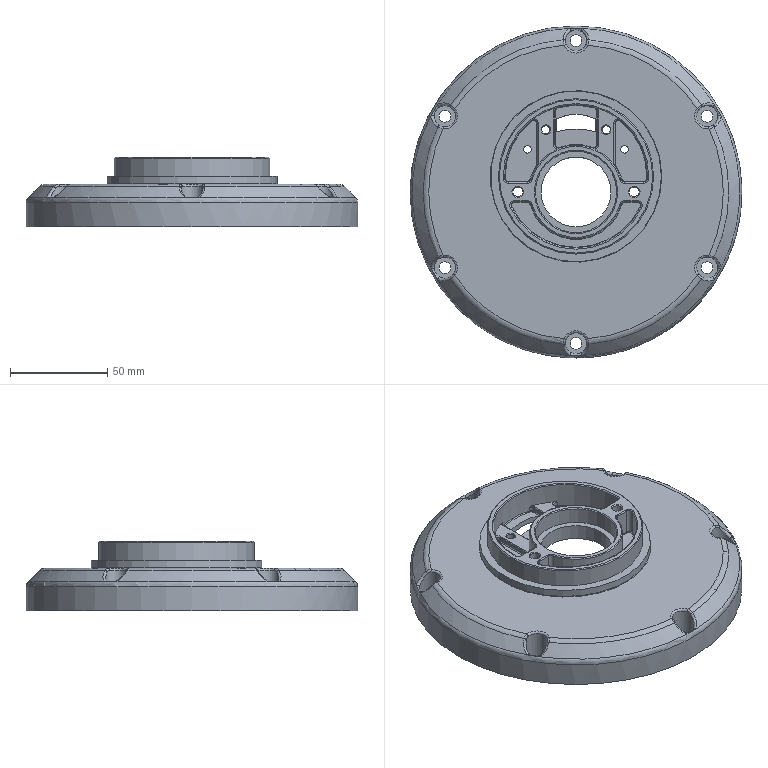NC program | NX | posted with a generic post | part box 171 x 171 x 36 mm
Lines 1 to 842 of 127321:
N10 G17 G21 G94 G90
(动态加工0.5 , TOOL : D12-L45)
N12 T01 M6
N14 G54
N16 G17 G0 G90 X-64.382 Y9.05 S4000 M3
N18 G43 Z20. H1
N20 Z-10.88
N22 G94 G1 X-64.242 Y8.994 Z-11.817 F2500.
N24 X-64.103 Y8.938 Z-12.188
N26 X-63.964 Y8.882 Z-12.46
N28 X-63.825 Y8.826 Z-12.68
N30 X-63.686 Y8.77 Z-12.864
N32 X-63.547 Y8.714 Z-13.022
N34 X-63.407 Y8.658 Z-13.16
N36 X-63.268 Y8.602 Z-13.28
N38 X-63.129 Y8.546 Z-13.385
N40 X-62.99 Y8.491 Z-13.478
N42 X-62.851 Y8.435 Z-13.559
N44 X-62.711 Y8.379 Z-13.63
N46 X-62.572 Y8.323 Z-13.69
N48 X-62.433 Y8.267 Z-13.742
N50 X-62.294 Y8.211 Z-13.785
N52 X-62.155 Y8.155 Z-13.819
N54 X-62.016 Y8.099 Z-13.846
N56 X-61.876 Y8.043 Z-13.865
N58 X-61.737 Y7.987 Z-13.876
N60 X-61.598 Y7.931 Z-13.88
N62 X-60.022 Y7.298
N64 G3 X-58.462 Y7.931 R1.212
N66 X-57.79 Y10.446 R18.547
N68 G2 X-54.48 Y21.711 R67.385
N70 X-58.367 Y5.726 R-58.65
N72 X-57.096 Y12.125 R73.511
N74 X-46.472 Y35.233 R59.829
N76 X-58.153 Y4.316 R-58.317
N78 X-56.825 Y11.882 R57.315
N80 X-48.098 Y32.386 R60.288
N82 X-12.022 Y56.727 R58.014
N84 X-8.455 Y57.479 R273.158
N86 G1 X-5.091 Y57.937
N88 G2 X3.976 Y58.038 R54.297
N90 G1 X6.985 Y57.708
N92 G2 X18.445 Y54.973 R73.242
N94 X-57.842 Y3.872 R-57.983
N96 X-55.833 Y14.511 R62.865
N98 X-18.954 Y54.458 R57.942
N100 G1 X-18.254 Y54.76
N102 X-15.051 Y55.886
N104 X-12.016 Y56.729
N106 G3 X-11.198 Y57.508 R1.201
N108 G1 X-11.078 Y57.872
N110 X-10.328 Y60.14 Z-13.68
N112 X-10.23 Y60.441 F15000.
N114 X-10.12 Y60.737
N116 G2 X-9.328 Y61.385 R1.202
N118 G1 X-8.364 Y61.628
N120 X-7.397 Y61.856
N122 G2 X-4.938 Y62.073 R11.089
N124 G1 X7.674 Y61.771
N126 G2 X8.813 Y60.846 R1.2
N128 G1 X8.915 Y60.412
N130 X9.462 Y58.086 Z-13.88 F2500.
N132 G3 X10.362 Y57.115 R1.222
N134 G1 X13.69 Y56.293
N136 G2 X25.715 Y51.6 R81.448
N138 X-57.571 Y2.84 R-57.649
N140 X-55.638 Y13.983 R58.924
N142 X-35.173 Y45.258 R57.932
N144 X-24.382 Y51.876 R57.646
N146 G1 X-21.373 Y53.419
N148 X-18.927 Y54.47
N150 G3 X-18.205 Y55.47 R1.201
N152 G1 X-18.21 Y55.716 Z-13.859
N154 X-18.241 Y55.961 Z-13.839
N156 X-18.482 Y57.841 Z-13.68
N158 X-18.526 Y58.166 F15000.
N160 X-18.554 Y58.492
N162 G2 X-17.535 Y59.663 R1.2
N164 G1 X-7.942 Y61.13
N166 G2 X0.222 Y61.787 R59.169
N168 X10.034 Y60.912 R44.909
N170 G1 X10.919 Y60.716
N172 X11.801 Y60.505
N174 X14.441 Y59.833
N176 G2 X15.272 Y59.083 R1.201
N178 G1 X15.332 Y58.916
N180 X16.155 Y56.673 Z-13.88 F2500.
N182 X16.446 Y55.879
N184 G3 X17.129 Y55.177 R1.202
N186 G1 X20.14 Y53.979
N188 G2 X28.502 Y49.735 R123.26
N190 X-57.274 Y1.986 R-57.318
N192 X-55.2 Y14.352 R57.763
N194 X-32.251 Y46.98 R57.521
N196 X-28.011 Y49.628 R63.272
N198 G1 X-27.303 Y50.121
N200 X-24.36 Y51.887
N202 G3 X-23.709 Y52.997 R1.201
N204 G1 X-23.714 Y53.14
N206 X-23.798 Y55.527 Z-13.68
N208 X-23.807 Y55.788 F15000.
N210 X-23.806 Y56.049
N212 G2 X-22.969 Y57.08 R1.2
N214 G1 X-15.131 Y59.529
N216 G2 X-9.06 Y61.038 R51.358
N218 X-1.947 Y61.731 R45.7
N220 X6.73 Y61.339 R57.035
N222 X11.815 Y60.431 R52.592
N224 X16.438 Y59.247 R80.834
N226 G1 X21.84 Y57.689
N228 G2 X22.707 Y56.502 R1.2
N230 G1 X22.695 Y56.082
N232 X22.627 Y53.693 Z-13.88 F2500.
N234 G3 X23.096 Y52.586 R1.249
N236 G2 X32.479 Y46.829 R128.559
N238 X-56.959 Y1.32 R-56.985
N240 X-54.768 Y14.686 R57.139
N242 X-31.191 Y47.294 R57.166
N244 X-27.996 Y49.638 R38.185
N246 G3 X-27.485 Y50.548 R1.202
N248 G1 X-27.444 Y51.221
N250 X-27.296 Y53.606 Z-13.68
N252 G2 X-27.222 Y54.134 R1.822 F15000.
N254 X-26.605 Y54.831 R1.202
N256 G1 X-24.444 Y55.87
N258 X-22.277 Y56.897
N260 G2 X-13.234 Y60.018 R52.406
N262 X-9.066 Y60.89 R58.164
N264 G1 X-2.445 Y62.019
N266 X-1.893 Y62.106
N268 X-1.339 Y62.178
N270 G2 X-0.227 Y62.167 R6.019
N272 G1 X3.977 Y61.712
N274 G2 X12.789 Y60.184 R87.371
N276 X19.994 Y57.966 R58.318
N278 G1 X21.096 Y57.536
N280 X22.191 Y57.088
N282 X24.917 Y55.938
N284 G2 X25.65 Y54.878 R1.201
N286 G1 X25.662 Y54.568
N288 X25.753 Y52.18 Z-13.88 F2500.
N290 X25.763 Y51.859
N292 X25.788 Y51.539
N294 G3 X26.309 Y50.745 R1.202
N296 G1 X29.076 Y48.918
N298 G3 X33.499 Y45.708 R391.88
N300 G2 X-47.695 Y-30.576 R-56.659
N302 X-56.593 Y1.961 R56.113
N304 X-52.891 Y19.404 R59.618
N306 X-33.943 Y44.941 R56.535
N308 X-31.185 Y47.298 R32.246
N310 G3 X-30.77 Y48.515 R1.201
N312 G1 X-30.952 Y49.031 Z-13.834
N314 X-31.15 Y49.541 Z-13.788
N316 X-31.61 Y50.752 Z-13.68
N318 X-31.72 Y51.038 F15000.
N320 X-31.817 Y51.328
N322 G2 X-31.185 Y52.674 R1.2
N324 G1 X-28.265 Y54.137
N326 X-25.337 Y55.585
N328 G2 X-16.872 Y58.981 R71.525
N330 G1 X-14.035 Y59.914
N332 X-11.19 Y60.817
N334 X-10.21 Y61.115
N336 X-9.224 Y61.394
N338 G2 X-5.372 Y61.829 R14.333
N340 G1 X1.344 Y61.672
N342 G2 X10.203 Y60.678 R50.544
N344 X13.603 Y59.945 R76.831
N346 X18.536 Y58.426 R50.135
N348 X22.978 Y56.686 R84.668
N350 G1 X29.672 Y53.839
N352 G2 X30.307 Y52.265 R1.2
N354 G1 X30.123 Y51.833
N356 X29.273 Y49.821 Z-13.863 F2500.
N358 X29.218 Y49.624 Z-13.88
N360 G3 X29.672 Y48.463 R1.201
N362 G2 X33.245 Y45.602 R52.943
N364 X40.55 Y39.085 R75.299
N366 X-56.307 Y0.098 R-56.317
N368 X-53.871 Y15.424 R56.258
N370 X-36.329 Y42.597 R56.623
N372 X-33.936 Y44.948 R26.685
N374 G3 X-33.6 Y46.177 R1.201
N376 G1 X-33.64 Y46.311
N378 X-34.33 Y48.598 Z-13.68
N380 X-34.408 Y48.856 F15000.
N382 X-34.475 Y49.117
N384 G2 X-33.936 Y50.324 R1.2
N386 G1 X-32.174 Y51.446
N388 X-30.406 Y52.559
N390 G2 X-26.258 Y54.918 R72.923
N392 X-22.263 Y56.931 R81.163
N394 X-17.932 Y58.708 R50.402
N396 X-13.848 Y59.891 R38.957
N398 X-10.21 Y60.685 R84.567
N400 X-3.569 Y61.538 R56.391
N402 G1 X-1.087 Y61.71
N404 X1.396 Y61.854
N406 G2 X3.383 Y61.89 R25.053
N408 X5.353 Y61.673 R14.115
N410 G1 X8.043 Y61.182
N412 X10.732 Y60.677
N414 G2 X16.674 Y59.069 R51.215
N416 X22.973 Y56.625 R66.107
N418 X26.528 Y54.851 R54.389
N420 G1 X32.534 Y51.57
N422 G2 X33.094 Y50.129 R1.2
N424 G1 X32.959 Y49.732
N426 X32.186 Y47.472 Z-13.88 F2500.
N428 G3 X32.534 Y46.194 R1.2
N430 G2 X35.672 Y43.312 R53.298
N432 X42.198 Y36.795 R78.841
N434 X-55.971 Y-0.703 R-55.983
N436 X-53.52 Y15.445 R55.574
N438 X-38.411 Y40.272 R56.447
N440 X-36.304 Y42.624 R25.471
N442 G3 X-36.006 Y43.723 R1.201
N444 G1 X-36.111 Y44.174
N446 X-36.655 Y46.5 Z-13.68
N448 X-36.708 Y46.727 F15000.
N450 X-36.75 Y46.957
N452 G2 X-36.304 Y48. R1.201
N454 G1 X-34.485 Y49.46
N456 X-32.654 Y50.907
N458 G2 X-27.198 Y54.454 R42.663
N460 X-19.772 Y57.923 R67.27
N462 X-8.298 Y61.017 R49.379
N464 G1 X-6.082 Y61.337
N466 X-3.862 Y61.623
N468 X-2.431 Y61.772
N470 X-0.997 Y61.886
N472 G2 X2.823 Y61.759 R22.036
N474 G1 X5.228 Y61.471
N476 X7.631 Y61.167
N478 G2 X15.261 Y59.498 R52.866
N480 G1 X16.792 Y59.042
N482 X18.313 Y58.553
N484 G2 X26.641 Y54.63 R43.392
N486 G1 X27.485 Y54.106
N488 X35.012 Y49.314
N490 G2 X35.522 Y47.974 R1.2
N492 G1 X35.429 Y47.647
N494 X34.777 Y45.348 Z-13.88 F2500.
N496 G3 X34.664 Y44.798 R2.051
N498 X35.012 Y43.938 R1.202
N500 G2 X37.986 Y40.838 R70.781
N502 X44.376 Y33.585 R75.525
N504 X-55.63 Y-1.011 R-55.65
N506 X-52.969 Y16.117 R55.524
N508 X-40.26 Y37.942 R56.258
N510 X-38.394 Y40.293 R31.284
N512 G3 X-38.138 Y41.276 R1.202
N514 G1 X-38.284 Y42.064
N516 X-38.719 Y44.414 Z-13.68
N518 G2 X-38.71 Y45.169 R1.407 F15000.
N520 X-38.394 Y45.669 R1.217
N522 G1 X-36.716 Y47.259
N524 X-35.027 Y48.837
N526 G2 X-30.056 Y52.627 R40.461
N528 X-25.642 Y55.258 R80.974
N530 X-20.582 Y57.605 R44.859
N532 X-17.192 Y58.876 R77.562
N534 X-12.072 Y60.304 R48.038
N536 X-3.912 Y61.724 R91.963
N538 X2.688 Y61.841 R34.231
N540 X12.242 Y60.346 R55.718
N542 G1 X13.763 Y59.968
N544 X15.28 Y59.578
N546 G2 X21.163 Y57.459 R42.183
N548 X28.705 Y53.543 R77.93
N550 X33.567 Y50.106 R37.117
N552 G1 X37.138 Y47.123
N554 G2 X37.543 Y45.954 R1.201
N556 G1 X37.49 Y45.701
N558 X36.995 Y43.364 Z-13.88 F2500.
N560 X36.913 Y42.996
N562 X36.849 Y42.625
N564 G3 X37.138 Y41.747 R1.203
N566 G2 X43.216 Y34.55 R340.95
N568 X-55.277 Y-1.824 R-55.32
N570 X-52.654 Y16.016 R54.877
N572 X-41.923 Y35.585 R56.207
N574 X-40.248 Y37.959 R50.636
N576 G3 X-40.163 Y39.223 R1.201
N578 G1 X-40.499 Y39.725 Z-13.829
N580 X-40.848 Y40.218 Z-13.779
N582 X-41.524 Y41.186 Z-13.68
N584 X-41.71 Y41.449 F15000.
N586 X-41.885 Y41.72
N588 G2 X-41.639 Y43.152 R1.2
N590 G1 X-40.413 Y44.296
N592 X-39.178 Y45.432
N594 G2 X-36.611 Y47.59 R56.207
N596 G1 X-34.679 Y49.119
N598 X-32.736 Y50.634
N600 G2 X-27.136 Y54.404 R58.023
N602 X-22.941 Y56.563 R47.75
N604 X-13.62 Y59.97 R58.737
N606 X-7.172 Y61.419 R72.619
N608 X0.821 Y61.908 R36.674
N610 G1 X2.406 Y61.831
N612 X3.99 Y61.744
N614 G2 X11.156 Y60.638 R45.158
N616 X23.345 Y56.439 R58.401
N618 X28.314 Y53.63 R45.247
N620 X34.421 Y49.356 R83.212
N622 G1 X40.453 Y44.716
N624 G2 X40.668 Y43.027 R1.2
N626 G1 X40.358 Y42.629
N628 X39.032 Y40.921 Z-13.861 F2500.
N630 X38.92 Y40.724 Z-13.88
N632 G3 X39.062 Y39.523 R1.201
N634 G1 X44.169 Y32.777
N636 G2 X-30.581 Y-45.696 R54.997
N638 X-54.956 Y-0.827 R54.797
N640 X-51.309 Y18.905 R55.779
N642 X-43.392 Y33.221 R55.66
N644 G1 X-41.908 Y35.609
N646 G3 X-41.935 Y36.919 R1.202
N648 G1 X-43.222 Y38.932 Z-13.68
N650 X-43.387 Y39.187 F15000.
N652 X-43.54 Y39.45
N654 G2 X-43.299 Y40.802 R1.2
N656 G1 X-40.794 Y43.313
N658 X-38.276 Y45.811
N660 G2 X-31.708 Y51.302 R62.48
N662 X-23.795 Y56.186 R54.707
N664 X-18.654 Y58.35 R44.203
N666 X-10.146 Y61.155 R202.654
N668 X-2.842 Y62.155 R23.271
N670 X0.969 Y62.023 R92.019
N672 X9.003 Y61.005 R61.91
N674 G1 X12.035 Y60.408
N676 G2 X16.944 Y59.019 R40.622
N678 X23.263 Y56.476 R75.097
N680 X27.714 Y53.991 R35.873
N682 X30.806 Y51.913 R92.185
N684 X36.047 Y47.743 R61.098
N686 G1 X42.494 Y42.007
N688 G2 X42.685 Y40.432 R1.2
N690 G1 X42.426 Y40.054
N692 X41.076 Y38.083 Z-13.88 F2500.
N694 G3 X41.102 Y36.814 R1.201
N696 X44.934 Y31.154 R169.581
N698 G2 X52.185 Y-16.238 R54.884
N700 X-54.573 Y-2.655 R54.643
N702 X-51.681 Y16.864 R54.346
N704 X-44.548 Y31.076 R55.865
N706 G1 X-43.388 Y33.227
N708 G3 X-43.369 Y34.462 R1.201
N710 G1 X-43.505 Y34.696
N712 X-44.704 Y36.763 Z-13.68
N714 X-44.832 Y36.985 F15000.
N716 X-44.952 Y37.212
N718 G2 X-44.78 Y38.42 R1.201
N720 G1 X-43.283 Y40.294
N722 X-41.773 Y42.159
N724 G2 X-37.357 Y46.766 R47.657
N726 X-34.649 Y49.174 R80.248
N728 X-26.763 Y54.589 R52.226
N730 X-19.637 Y58.021 R66.873
N732 X-14.541 Y59.77 R44.941
N734 X-11.327 Y60.512 R47.008
N736 X-3.951 Y61.497 R53.567
N738 G1 X1.27 Y61.826
N740 G2 X7.182 Y61.46 R23.857
N742 X11.566 Y60.557 R81.836
N744 X17.187 Y58.919 R67.452
N746 X22.108 Y56.903 R47.835
N748 G1 X23.563 Y56.209
N750 X25.014 Y55.507
N752 G2 X30.744 Y52.107 R46.484
N754 X34.085 Y49.477 R38.994
N756 X37.561 Y46.362 R143.152
N758 X41.224 Y42.703 R83.07
N760 G1 X43.885 Y39.871
N762 G2 X44.025 Y38.407 R1.2
N764 G1 X43.841 Y38.116
N766 X42.563 Y36.097 Z-13.88 F2500.
N768 G3 X42.323 Y35.098 R1.287
N770 X42.494 Y34.678 R1.268
N772 G2 X43.848 Y32.395 R32.787
N774 X47.676 Y26.035 R127.693
N776 X-54.204 Y-3.285 R-54.314
N778 X-51.281 Y17.007 R53.899
N780 X-45.635 Y28.842 R56.01
N782 X-44.537 Y31.098 R21.208
N784 G3 X-44.541 Y32.231 R1.201
N786 G1 X-44.791 Y32.694
N788 X-45.926 Y34.797 Z-13.68
N790 G2 X-46.141 Y35.276 R1.873 F15000.
N792 X-45.928 Y36.29 R1.202
N794 G1 X-43.55 Y39.404
N796 X-41.159 Y42.507
N798 G2 X-38.508 Y45.638 R58.282
N800 X-35.783 Y48.172 R25.901
N802 G1 X-33.981 Y49.62
N804 X-32.157 Y51.04
N806 G2 X-28.548 Y53.614 R72.72
N808 X-23.406 Y56.395 R36.796
N810 X-12.371 Y60.248 R60.482
N812 X-7.337 Y61.239 R73.589
N814 X-1.86 Y61.921 R69.047
N816 X3.342 Y61.848 R30.057
N818 X11.422 Y60.493 R53.98
N820 G1 X13.304 Y60.025
N822 X15.183 Y59.545
N824 G2 X22.706 Y56.716 R44.767
N826 X31.085 Y51.88 R55.876
N828 X38.725 Y45.253 R49.144
N830 X41.899 Y41.69 R77.926
N832 G1 X45.022 Y37.956
N834 G2 X45.145 Y36.592 R1.2
N836 G1 X44.999 Y36.336
N838 X43.817 Y34.259 Z-13.88 F2500.
N840 X43.689 Y34.033
N842 X43.569 Y33.803
N844 G3 X43.631 Y32.763 R1.202
N846 G2 X45.421 Y29.447 R107.163
N848 X49.426 Y21.709 R83.06
N850 X-53.847 Y-3.609 R-53.978
N852 X-50.779 Y17.439 R53.624
N854 X-46.631 Y26.547 R56.86
N856 X-45.629 Y28.856 R31.273
N858 G3 X-45.78 Y30.087 R1.201
N860 X-46.211 Y30.455 Z-13.832 R1.918
N862 G1 X-47.692 Y31.513 Z-13.68
N864 X-47.951 Y31.695 F15000.
N866 X-48.202 Y31.89
N868 G2 X-48.317 Y33.512 R1.2
N870 G1 X-41.335 Y42.264
N872 G2 X-37.913 Y46.208 R60.363
N874 X-35.146 Y48.697 R27.278
N876 G1 X-33.032 Y50.354
N878 X-30.908 Y51.998
N880 G2 X-23.997 Y56.081 R38.348
N882 G1 X-21.053 Y57.42
N884 G2 X-11.609 Y60.436 R48.414
N886 X-5.634 Y61.469 R111.059
N888 X-2.417 Y61.846 R66.098
N890 X2.682 Y61.847 R31.155
N892 X10.784 Y60.638 R53.314
N894 G1 X12.357 Y60.274
N896 X13.927 Y59.899
N898 G2 X19.359 Y58.141 R47.657
N900 X25.077 Y55.604 R54.598
N902 X31.125 Y51.794 R46.144
N904 X37.01 Y47.047 R76.829
N906 X40.538 Y43.357 R37.204
N908 X44.587 Y38.12 R70.632
N910 G1 X46.179 Y35.835
N912 G2 X46.267 Y34.61 R1.201
N914 G1 X46.16 Y34.397
N916 X45.087 Y32.262 Z-13.88 F2500.
N918 X44.907 Y31.909
N920 X44.74 Y31.55
N922 G3 X44.788 Y30.642 R1.203
N924 X48.263 Y23.476 R353.472
N926 G2 X27.875 Y-45.834 R53.726
N928 X-53.537 Y-3.106 R53.61
N930 X-49.927 Y18.788 R53.703
N932 X-47.446 Y24.335 R58.379
N934 G1 X-46.629 Y26.552
N936 G3 X-46.858 Y27.764 R1.201
N938 G1 X-47.102 Y27.985 Z-13.852
N940 X-47.36 Y28.19 Z-13.825
N942 X-48.706 Y29.277 Z-13.68
N944 X-48.962 Y29.48 F15000.
N946 X-49.208 Y29.696
N948 G2 X-49.317 Y31.208 R1.2
N950 G1 X-42.462 Y40.988
N952 X-41.456 Y42.41
N954 X-40.425 Y43.813
N956 G2 X-38.731 Y45.62 R14.172
N958 X-34.889 Y48.927 R89.543
N960 X-30.194 Y52.44 R97.268
N962 X-15.927 Y59.306 R51.086
N964 X-7.965 Y61.264 R69.034
N966 G1 X-5.68 Y61.668
N968 G2 X0.907 Y62.01 R32.297
N970 X8.299 Y61.098 R51.697
N972 G1 X10.545 Y60.657
N974 X12.789 Y60.202
N976 G2 X18.396 Y58.545 R42.577
N978 X23.35 Y56.491 R52.691
N980 X27.128 Y54.398 R40.747
N982 X32.894 Y50.513 R72.413
N984 X36.93 Y47.044 R43.562
N986 X43.853 Y39.194 R61.331
N988 G1 X48.794 Y32.502
N990 G2 X48.564 Y30.841 R1.2
N992 G1 X48.17 Y30.535
N994 X46.439 Y29.189 Z-13.864 F2500.
N996 X46.301 Y29.05 Z-13.88
N998 G3 X46.106 Y27.847 R1.201
N1000 X48.413 Y22.428 R83.307
N1002 G2 X53.24 Y-2.822 R54.429
N1004 X-53.13 Y-4.202 R53.304
N1006 X-49.839 Y18.074 R53.047
N1008 X-48.103 Y22.243 R66.624
N1010 X-47.44 Y24.352 R21.473
N1012 G3 X-47.751 Y25.647 R1.2
N1014 G1 X-49.568 Y27.199 Z-13.68
N1016 X-49.791 Y27.387 F15000.
N1018 X-50.004 Y27.587
N1020 G2 X-50.128 Y29.008 R1.2
N1022 G1 X-46.228 Y35.374
N1024 G2 X-41.008 Y42.62 R59.842
N1026 G1 X-40. Y43.82
N1028 X-38.982 Y45.012
N1030 G2 X-33.022 Y50.379 R35.346
N1032 G1 X-31.159 Y51.711
N1034 X-29.287 Y53.03
N1036 G2 X-24.896 Y55.625 R39.989
N1038 X-17.958 Y58.725 R79.057
N1040 X-12.828 Y60.279 R39.404
N1042 X-4.82 Y61.569 R63.326
N1044 X2.884 Y61.852 R77.28
N1046 X8.054 Y61.269 R29.867
N1048 G1 X9.67 Y60.942
N1050 X11.284 Y60.605
N1052 G2 X22.365 Y56.883 R57.14
N1054 X26.465 Y54.852 R66.788
N1056 X30.694 Y52.19 R43.933
N1058 X35.618 Y48.33 R52.097
N1060 X38.075 Y45.939 R47.264
N1062 X42.443 Y40.855 R54.248
N1064 X46.787 Y34.798 R101.44
N1066 G1 X49.49 Y30.721
N1068 G2 X49.247 Y29.127 R1.2
N1070 G1 X48.936 Y28.875
N1072 X47.085 Y27.364 Z-13.88 F2500.
N1074 G3 X46.802 Y26.065 R1.2
N1076 G2 X47.889 Y23.088 R67.08
N1078 X50.558 Y15.841 R101.281
N1080 X-52.746 Y-4.756 R-52.972
N1082 X-49.522 Y17.969 R52.618
N1084 G1 X-48.718 Y20.036
N1086 G2 X-48.099 Y22.259 R26.226
N1088 G3 X-48.425 Y23.468 R1.201
N1090 G1 X-48.557 Y23.594
N1092 X-50.293 Y25.236 Z-13.68
N1094 X-50.479 Y25.413 F15000.
N1096 X-50.657 Y25.596
N1098 G2 X-50.787 Y26.915 R1.2
N1100 G1 X-49.091 Y30.119
N1102 X-47.382 Y33.316
N1104 G2 X-42.881 Y40.594 R82.24
N1106 X-37.577 Y46.588 R37.337
N1108 X-33.766 Y49.933 R88.866
N1110 X-31.208 Y51.92 R60.821
N1112 X-26.867 Y54.603 R35.035
N1114 X-22.327 Y56.859 R86.503
N1116 X-17.78 Y58.738 R75.645
N1118 X-12.643 Y60.28 R41.442
N1120 G1 X-11.768 Y60.463
N1122 X-10.889 Y60.627
N1124 G2 X-5.727 Y61.42 R96.476
N1126 X-1.085 Y61.829 R69.005
N1128 X6.474 Y61.463 R40.58
N1130 X12.732 Y60.197 R52.09
N1132 G1 X14.291 Y59.781
N1134 X15.847 Y59.353
N1136 G2 X25.015 Y55.571 R47.155
N1138 X34.878 Y48.902 R61.279
N1140 X39.812 Y44.023 R38.272
N1142 X42.174 Y41.143 R91.014
N1144 X45.984 Y35.635 R60.384
N1146 G1 X50.232 Y28.701
N1148 G2 X50.005 Y27.176 R1.2
N1150 G1 X49.701 Y26.907
N1152 X47.914 Y25.321 Z-13.88 F2500.
N1154 G3 X47.544 Y24.045 R1.202
N1156 X49.946 Y16.716 R264.689
N1158 G2 X40.223 Y-33.954 R52.829
N1160 X-52.432 Y-4.452 R52.616
N1162 X-49.191 Y17.903 R52.422
N1164 G1 X-48.712 Y20.063
N1166 G3 X-49.015 Y21.15 R1.201
N1168 G1 X-49.292 Y21.441
N1170 X-50.941 Y23.17 Z-13.68
N1172 X-51.109 Y23.346 F15000.
N1174 X-51.27 Y23.529
N1176 G2 X-51.4 Y24.719 R1.201
N1178 G1 X-50.263 Y27.316
N1180 X-49.113 Y29.907
N1182 G2 X-46.472 Y35.028 R63.685
N1184 X-43.732 Y39.166 R43.348
N1186 X-40.622 Y43.172 R93.752
N1188 X-38.495 Y45.614 R62.833
N1190 X-34.747 Y49.076 R34.446
N1192 X-31.198 Y51.798 R81.141
N1194 X-26.538 Y54.771 R49.554
N1196 X-23.496 Y56.293 R41.37
N1198 G1 X-21.989 Y56.97
N1200 X-20.476 Y57.636
N1202 G2 X-12.383 Y60.239 R49.492
N1204 X-7.15 Y61.203 R57.866
N1206 G1 X-5.262 Y61.464
N1208 X-3.371 Y61.71
N1210 G2 X4.293 Y61.744 R36.431
N1212 X11.801 Y60.443 R51.95
N1214 X18.636 Y58.391 R69.831
N1216 X24.568 Y55.722 R44.382
N1218 X29.109 Y53.149 R88.453
N1220 X32.904 Y50.634 R63.587
N1222 X37.843 Y46.259 R34.586
N1224 G1 X38.945 Y45.077
N1226 X40.04 Y43.888
N1228 G2 X43.59 Y39.418 R50.669
N1230 X46.54 Y35.107 R91.699
N1232 X48.328 Y31.839 R31.701
N1234 G1 X51.068 Y26.038
N1236 G2 X50.838 Y24.683 R1.2
N1238 G1 X50.577 Y24.419
N1240 X48.901 Y22.717 Z-13.88 F2500.
N1242 X48.592 Y22.389
N1244 G3 X48.38 Y21.382 R1.202
N1246 X49.882 Y15.914 R70.407
N1248 G2 X52.096 Y-4.688 R54.185
N1250 X-52.03 Y-5.17 R52.295
N1252 X-49.54 Y15.922 R51.903
N1254 X-49.179 Y17.95 R19.221
N1256 G3 X-49.46 Y19.013 R1.201
N1258 G1 X-49.896 Y19.497
N1260 X-51.496 Y21.272 Z-13.68
N1262 G2 X-51.866 Y21.822 R1.547 F15000.
N1264 X-51.867 Y22.606 R1.206
N1266 G1 X-51.223 Y24.487
N1268 X-50.566 Y26.363
N1270 G2 X-48.278 Y31.595 R49.16
N1272 X-44.524 Y38.023 R53.246
N1274 X-41.083 Y42.901 R128.742
N1276 X-38.105 Y46.224 R24.854
N1278 G1 X-36.924 Y47.326
N1280 X-35.733 Y48.418
N1282 G2 X-29.342 Y53.101 R42.17
N1284 X-26.124 Y54.97 R81.731
N1286 X-17.961 Y58.58 R57.009
N1288 X-9.898 Y60.906 R71.59
N1290 X-0.524 Y61.826 R39.168
N1292 G1 X1.437 Y61.785
N1294 X3.398 Y61.727
N1296 G2 X9.845 Y60.887 R39.216
N1298 X17.034 Y58.938 R71.534
N1300 G1 X19.298 Y58.184
N1302 G2 X24.208 Y56.034 R39.736
N1304 X29.72 Y52.77 R58.817
N1306 X36.775 Y47.119 R60.737
N1308 X40.854 Y42.924 R64.748
N1310 X46.475 Y35.057 R48.375
N1312 X50.384 Y27.022 R58.657
N1314 G1 X51.514 Y24.178
N1316 G2 X51.273 Y22.912 R1.201
N1318 G1 X51.104 Y22.734
N1320 X49.467 Y20.994 Z-13.88 F2500.
N1322 X49.241 Y20.756
N1324 X49.024 Y20.511
N1326 G3 X48.826 Y19.522 R1.202
N1328 G2 X49.486 Y16.52 R76.464
N1330 X51.198 Y8.954 R104.119
N1332 X-51.62 Y-5.851 R-51.963
N1334 X-49.862 Y13.762 R51.39
N1336 G1 X-49.537 Y15.938
N1338 G3 X-50.016 Y17.086 R1.201
N1340 X-50.504 Y17.32 Z-13.835 R1.995
N1342 G1 X-52.225 Y17.989 Z-13.68
N1344 X-52.52 Y18.102 F15000.
N1346 X-52.81 Y18.228
N1348 G2 X-53.339 Y19.74 R1.2
N1350 G1 X-49.899 Y28.011
N1352 G2 X-46.875 Y34.273 R61.922
N1354 X-43.78 Y39.07 R48.455
N1356 X-38.493 Y45.571 R66.636
N1358 X-33.645 Y49.906 R37.597
N1360 G1 X-31.053 Y51.836
N1362 G2 X-25.419 Y55.397 R52.411
N1364 X-21.574 Y57.213 R40.83
N1366 X-17.056 Y58.974 R89.502
N1368 X-10.147 Y61.003 R71.301
N1370 X-0.704 Y61.974 R37.002
N1372 X8.923 Y61.023 R58.773
N1374 X12.336 Y60.351 R81.394
N1376 X21.722 Y57.16 R47.429
N1378 X29.955 Y52.568 R54.755
N1380 X35.695 Y48.315 R73.306
N1382 X40.283 Y43.715 R36.206
N1384 X44.99 Y37.375 R59.822
N1386 X47.877 Y32.548 R73.046
N1388 X49.937 Y27.88 R34.191
N1390 G1 X51.956 Y22.186
N1392 G2 X51.725 Y20.992 R1.201
N1394 G1 X51.599 Y20.849
N1396 X50.02 Y19.056 Z-13.88 F2500.
N1398 X49.733 Y18.734
N1400 X49.457 Y18.403
N1402 G3 X49.268 Y17.531 R1.203
N1404 X50.582 Y10.551 R143.399
N1406 G2 X47.084 Y-21.182 R52.23
N1408 X-51.315 Y-5.512 R51.612
N1410 X-50.019 Y11.865 R50.599
N1412 G1 X-49.862 Y13.771
N1414 G3 X-50.392 Y14.868 R1.201
N1416 G1 X-50.684 Y15.021 Z-13.852
N1418 X-50.986 Y15.153 Z-13.825
N1420 X-52.564 Y15.863 Z-13.68
N1422 X-52.87 Y15.998 F15000.
N1424 X-53.17 Y16.148
N1426 G2 X-53.663 Y17.572 R1.2
N1428 G1 X-50.625 Y26.002
N1430 G2 X-47.425 Y33.268 R56.082
N1432 X-45.401 Y36.684 R46.069
N1434 X-42.55 Y40.88 R89.403
N1436 X-40.573 Y43.445 R58.623
N1438 X-37.009 Y47.091 R31.539
N1440 X-34.171 Y49.501 R86.465
N1442 X-28.715 Y53.384 R57.594
N1444 X-25.745 Y55.192 R72.066
N1446 X-16.618 Y59.05 R44.098
N1448 G1 X-15.101 Y59.499
N1450 X-13.581 Y59.94
N1452 G2 X-7.195 Y61.204 R45.229
N1454 X1.067 Y61.839 R85.918
N1456 X7.642 Y61.323 R34.71
N1458 X17.512 Y58.836 R70.837
N1460 X23.897 Y56.104 R47.642
N1462 X28.218 Y53.652 R71.307
N1464 X34.106 Y49.613 R66.462
N1466 X38.844 Y45.164 R36.254
N1468 G1 X39.917 Y43.957
N1470 X40.982 Y42.745
N1472 G2 X47.135 Y33.735 R51.255
N1474 X50.579 Y26.304 R59.171
N1476 G1 X53.553 Y18.469
N1478 G2 X52.907 Y16.942 R1.2
N1480 G1 X52.457 Y16.747
N1482 X50.369 Y15.839 Z-13.871 F2500.
N1484 X50.273 Y15.78 Z-13.88
N1486 G3 X49.751 Y14.668 R1.201
N1488 X50.463 Y9.557 R56.897
N1490 G2 X50.534 Y-8.802 R53.895
N1492 X-50.924 Y-5.981 R51.281
N1494 X-50.146 Y9.834 R50.239
N1496 X-50.016 Y11.899 R20.864
N1498 G3 X-50.67 Y13.068 R1.2
N1500 G1 X-52.825 Y14.1 Z-13.68
N1502 X-53.075 Y14.22 F15000.
N1504 X-53.321 Y14.349
N1506 G2 X-53.818 Y15.7 R1.2
N1508 G1 X-51.246 Y24.28
N1510 G2 X-48.638 Y30.928 R44.816
N1512 X-45.365 Y36.833 R57.798
N1514 X-42.613 Y40.663 R47.975
N1516 X-37.173 Y46.902 R72.155
N1518 X-32.091 Y51.118 R35.269
N1520 G1 X-30.475 Y52.222
N1522 X-28.852 Y53.316
N1524 G2 X-21.221 Y57.357 R48.165
N1526 X-12.122 Y60.287 R56.277
N1528 X-7.524 Y61.188 R81.925
N1530 X-2.465 Y61.952 R91.699
N1532 X1.355 Y62.003 R21.278
N1534 X4.964 Y61.682 R81.872
N1536 X10.213 Y60.799 R53.633
N1538 G1 X11.79 Y60.453
N1540 X13.365 Y60.094
N1542 G2 X18.809 Y58.387 R46.66
N1544 X24.538 Y55.872 R50.834
N1546 X26.87 Y54.548 R41.631
N1548 X30.026 Y52.563 R90.563
N1550 X33.289 Y50.208 R48.809
N1552 X35.321 Y48.459 R37.929
N1554 G1 X36.76 Y47.128
N1556 X38.188 Y45.786
N1558 G2 X42.956 Y40.324 R44.872
N1560 X48.952 Y30.054 R49.1
N1562 X51.893 Y22.407 R87.825
N1564 G1 X53.705 Y16.939
N1566 G2 X53.063 Y15.47 R1.2
N1568 G1 X52.699 Y15.304
N1570 X50.526 Y14.311 Z-13.88 F2500.
N1572 G3 X49.903 Y13.138 R1.2
N1574 X50.297 Y8.991 R405.418
N1576 G2 X50.947 Y-1.133 R66.628
N1578 X-50.516 Y-6.535 R50.947
N1580 X-50.175 Y7.847 R49.411
N1582 G1 X-50.146 Y9.835
N1584 G3 X-50.766 Y10.903 R1.201
N1586 G1 X-50.898 Y10.976
N1588 X-52.991 Y12.13 Z-13.68
N1590 X-53.24 Y12.266 F15000.
N1592 X-53.484 Y12.413
N1594 G2 X-53.947 Y13.636 R1.201
N1596 G1 X-53.051 Y17.715
N1598 G2 X-50.979 Y25.07 R84.132
N1600 X-48.703 Y30.688 R55.739
N1602 X-44.259 Y38.436 R48.366
N1604 X-42.453 Y40.807 R45.979
N1606 G1 X-40.981 Y42.615
N1608 X-39.495 Y44.411
N1610 G2 X-34.837 Y48.939 R36.425
N1612 X-31.912 Y51.252 R83.237
N1614 X-25.618 Y55.23 R47.822
N1616 X-20.22 Y57.743 R47.926
N1618 G1 X-18.599 Y58.377
N1620 X-16.965 Y58.978
N1622 G2 X-13.168 Y60.146 R53.67
N1624 X-7.367 Y61.55 R130.36
N1626 X-1.463 Y62.082 R23.935
N1628 X2.263 Y61.91 R83.964
N1630 X8.899 Y61.013 R55.959
N1632 G1 X10.606 Y60.677
N1634 X12.307 Y60.306
N1636 G2 X23.514 Y56.312 R52.545
N1638 X27.641 Y54.027 R52.778
N1640 X33.727 Y49.75 R51.189
N1642 G1 X34.998 Y48.71
N1644 X36.248 Y47.646
N1646 G2 X40.641 Y43.204 R42.97
N1648 X45.193 Y37.117 R65.267
N1650 X50.462 Y26.457 R49.089
N1652 X52.9 Y18.631 R97.05
N1654 G1 X53.898 Y14.87
N1656 G2 X53.292 Y13.498 R1.2
N1658 G1 X52.91 Y13.299
N1660 X50.791 Y12.196 Z-13.88 F2500.
N1662 G3 X50.096 Y11.069 R1.204
N1664 X50.482 Y4.329 R101.857
N1666 G2 X45.636 Y-21.894 R51.569
N1668 X-50.236 Y-6.017 R50.596
N1670 X-50.129 Y5.939 R49.605
N1672 X-50.175 Y7.872 R18.316
N1674 G3 X-50.776 Y8.929 R1.201
N1676 G1 X-51.052 Y9.089
N1678 X-53.123 Y10.281 Z-13.68
N1680 X-53.327 Y10.399 F15000.
N1682 X-53.526 Y10.526